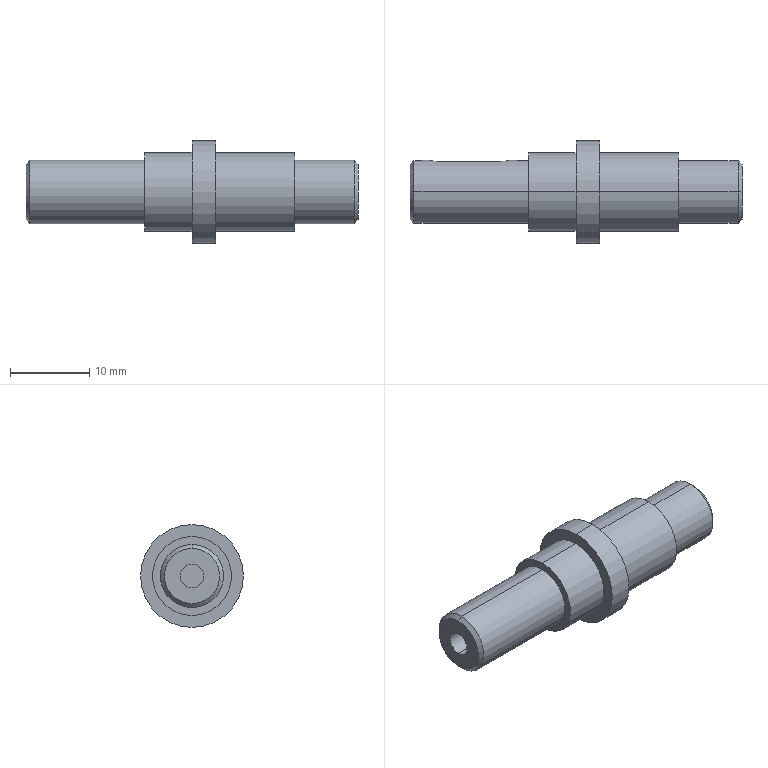Part | SolidWorks | features Chamfer 2, ICE 2, Revolution 1 | 1 solid | 28 faces | box 42 x 13 x 13 mm | volume 2716 mm3 | cylinder 14 | plane 10 | cone 4 | commonest cylinder face diameters 8 x4 10 x4 2 x2 3 x2 13 x2
STEP:
#1=CARTESIAN_POINT('',(18.732,0.,-3.5));
#2=VERTEX_POINT('',#1);
#3=CARTESIAN_POINT('',(18.732,0.,3.5));
#4=VERTEX_POINT('',#3);
#5=CARTESIAN_POINT('',(18.732,0.,0.));
#6=DIRECTION('',(1.,0.,0.));
#7=DIRECTION('',(0.,0.,1.));
#8=AXIS2_PLACEMENT_3D('',#5,#6,#7);
#9=CIRCLE('',#8,3.5);
#10=EDGE_CURVE('',#2,#4,#9,.T.);
#11=ORIENTED_EDGE('',*,*,#10,.F.);
#12=CARTESIAN_POINT('',(18.232,0.,-4.));
#13=VERTEX_POINT('',#12);
#14=CARTESIAN_POINT('',(18.232,0.,-4.));
#15=DIRECTION('',(-0.7071,0.,-0.7071));
#16=VECTOR('',#15,1000.);
#17=LINE('',#14,#16);
#18=EDGE_CURVE('',#2,#13,#17,.T.);
#19=ORIENTED_EDGE('',*,*,#18,.T.);
#20=CARTESIAN_POINT('',(18.232,0.,4.));
#21=VERTEX_POINT('',#20);
#22=CARTESIAN_POINT('',(18.232,0.,0.));
#23=DIRECTION('',(-1.,0.,0.));
#24=DIRECTION('',(0.,0.,1.));
#25=AXIS2_PLACEMENT_3D('',#22,#23,#24);
#26=CIRCLE('',#25,4.);
#27=EDGE_CURVE('',#21,#13,#26,.T.);
#28=ORIENTED_EDGE('',*,*,#27,.F.);
#29=CARTESIAN_POINT('',(18.232,0.,4.));
#30=DIRECTION('',(-0.7071,0.,0.7071));
#31=VECTOR('',#30,1000.);
#32=LINE('',#29,#31);
#33=EDGE_CURVE('',#4,#21,#32,.T.);
#34=ORIENTED_EDGE('',*,*,#33,.F.);
#35=EDGE_LOOP('',(#11,#19,#28,#34));
#36=FACE_OUTER_BOUND('',#35,.T.);
#37=CARTESIAN_POINT('',(18.232,0.,0.));
#38=DIRECTION('',(-1.,0.,0.));
#39=DIRECTION('',(0.,0.,1.));
#40=AXIS2_PLACEMENT_3D('',#37,#38,#39);
#41=CONICAL_SURFACE('',#40,4.,0.7854);
#42=ADVANCED_FACE('',(#36),#41,.T.);
#43=CARTESIAN_POINT('',(-23.268,0.,3.5));
#44=VERTEX_POINT('',#43);
#45=CARTESIAN_POINT('',(-23.268,0.,-3.5));
#46=VERTEX_POINT('',#45);
#47=CARTESIAN_POINT('',(-23.268,0.,0.));
#48=DIRECTION('',(-1.,0.,0.));
#49=DIRECTION('',(0.,0.,-1.));
#50=AXIS2_PLACEMENT_3D('',#47,#48,#49);
#51=CIRCLE('',#50,3.5);
#52=EDGE_CURVE('',#44,#46,#51,.T.);
#53=ORIENTED_EDGE('',*,*,#52,.F.);
#54=CARTESIAN_POINT('',(-22.768,0.,4.));
#55=VERTEX_POINT('',#54);
#56=CARTESIAN_POINT('',(-23.268,0.,3.5));
#57=DIRECTION('',(0.7071,0.,0.7071));
#58=VECTOR('',#57,1000.);
#59=LINE('',#56,#58);
#60=EDGE_CURVE('',#44,#55,#59,.T.);
#61=ORIENTED_EDGE('',*,*,#60,.T.);
#62=CARTESIAN_POINT('',(-22.768,0.,-4.));
#63=VERTEX_POINT('',#62);
#64=CARTESIAN_POINT('',(-22.768,0.,0.));
#65=DIRECTION('',(1.,0.,0.));
#66=DIRECTION('',(0.,0.,-1.));
#67=AXIS2_PLACEMENT_3D('',#64,#65,#66);
#68=CIRCLE('',#67,4.);
#69=EDGE_CURVE('',#63,#55,#68,.T.);
#70=ORIENTED_EDGE('',*,*,#69,.F.);
#71=CARTESIAN_POINT('',(-23.268,0.,-3.5));
#72=DIRECTION('',(0.7071,0.,-0.7071));
#73=VECTOR('',#72,1000.);
#74=LINE('',#71,#73);
#75=EDGE_CURVE('',#46,#63,#74,.T.);
#76=ORIENTED_EDGE('',*,*,#75,.F.);
#77=EDGE_LOOP('',(#53,#61,#70,#76));
#78=FACE_OUTER_BOUND('',#77,.T.);
#79=CARTESIAN_POINT('',(-23.268,0.,0.));
#80=DIRECTION('',(1.,0.,0.));
#81=DIRECTION('',(0.,0.,-1.));
#82=AXIS2_PLACEMENT_3D('',#79,#80,#81);
#83=CONICAL_SURFACE('',#82,3.5,0.7854);
#84=ADVANCED_FACE('',(#78),#83,.T.);
#85=CARTESIAN_POINT('',(-13.268,0.,-1.5));
#86=VERTEX_POINT('',#85);
#87=CARTESIAN_POINT('',(-13.268,0.,1.5));
#88=VERTEX_POINT('',#87);
#89=CARTESIAN_POINT('',(-13.268,0.,0.));
#90=DIRECTION('',(-1.,0.,0.));
#91=DIRECTION('',(0.,0.,1.));
#92=AXIS2_PLACEMENT_3D('',#89,#90,#91);
#93=CIRCLE('',#92,1.5);
#94=EDGE_CURVE('',#86,#88,#93,.T.);
#95=ORIENTED_EDGE('',*,*,#94,.F.);
#96=CARTESIAN_POINT('',(-23.268,0.,-1.5));
#97=VERTEX_POINT('',#96);
#98=CARTESIAN_POINT('',(-13.268,0.,-1.5));
#99=DIRECTION('',(-1.,0.,0.));
#100=VECTOR('',#99,1000.);
#101=LINE('',#98,#100);
#102=EDGE_CURVE('',#86,#97,#101,.T.);
#103=ORIENTED_EDGE('',*,*,#102,.T.);
#104=CARTESIAN_POINT('',(-23.268,0.,1.5));
#105=VERTEX_POINT('',#104);
#106=CARTESIAN_POINT('',(-23.268,0.,0.));
#107=DIRECTION('',(-1.,0.,0.));
#108=DIRECTION('',(0.,0.,1.));
#109=AXIS2_PLACEMENT_3D('',#106,#107,#108);
#110=CIRCLE('',#109,1.5);
#111=EDGE_CURVE('',#97,#105,#110,.T.);
#112=ORIENTED_EDGE('',*,*,#111,.T.);
#113=CARTESIAN_POINT('',(-13.268,0.,1.5));
#114=DIRECTION('',(-1.,0.,0.));
#115=VECTOR('',#114,1000.);
#116=LINE('',#113,#115);
#117=EDGE_CURVE('',#88,#105,#116,.T.);
#118=ORIENTED_EDGE('',*,*,#117,.F.);
#119=EDGE_LOOP('',(#95,#103,#112,#118));
#120=FACE_OUTER_BOUND('',#119,.T.);
#121=CARTESIAN_POINT('',(-13.268,0.,0.));
#122=DIRECTION('',(-1.,0.,0.));
#123=DIRECTION('',(0.,0.,1.));
#124=AXIS2_PLACEMENT_3D('',#121,#122,#123);
#125=CYLINDRICAL_SURFACE('',#124,1.5);
#126=ADVANCED_FACE('',(#120),#125,.F.);
#127=ORIENTED_EDGE('',*,*,#27,.T.);
#128=CARTESIAN_POINT('',(10.732,0.,-4.));
#129=VERTEX_POINT('',#128);
#130=CARTESIAN_POINT('',(-82.031,0.,-4.));
#131=DIRECTION('',(-1.,0.,0.));
#132=VECTOR('',#131,1000.);
#133=LINE('',#130,#132);
#134=EDGE_CURVE('',#13,#129,#133,.T.);
#135=ORIENTED_EDGE('',*,*,#134,.T.);
#136=CARTESIAN_POINT('',(10.732,0.,4.));
#137=VERTEX_POINT('',#136);
#138=CARTESIAN_POINT('',(10.732,0.,0.));
#139=DIRECTION('',(-1.,0.,0.));
#140=DIRECTION('',(0.,0.,1.));
#141=AXIS2_PLACEMENT_3D('',#138,#139,#140);
#142=CIRCLE('',#141,4.);
#143=EDGE_CURVE('',#137,#129,#142,.T.);
#144=ORIENTED_EDGE('',*,*,#143,.F.);
#145=CARTESIAN_POINT('',(-82.031,0.,4.));
#146=DIRECTION('',(-1.,0.,0.));
#147=VECTOR('',#146,1000.);
#148=LINE('',#145,#147);
#149=EDGE_CURVE('',#21,#137,#148,.T.);
#150=ORIENTED_EDGE('',*,*,#149,.F.);
#151=EDGE_LOOP('',(#127,#135,#144,#150));
#152=FACE_OUTER_BOUND('',#151,.T.);
#153=CARTESIAN_POINT('',(-82.031,0.,0.));
#154=DIRECTION('',(-1.,0.,0.));
#155=DIRECTION('',(0.,0.,1.));
#156=AXIS2_PLACEMENT_3D('',#153,#154,#155);
#157=CYLINDRICAL_SURFACE('',#156,4.);
#158=ADVANCED_FACE('',(#152),#157,.T.);
#159=CARTESIAN_POINT('',(10.732,0.,5.));
#160=VERTEX_POINT('',#159);
#161=CARTESIAN_POINT('',(10.732,0.,-5.));
#162=VERTEX_POINT('',#161);
#163=CARTESIAN_POINT('',(10.732,0.,0.));
#164=DIRECTION('',(-1.,0.,0.));
#165=DIRECTION('',(0.,0.,1.));
#166=AXIS2_PLACEMENT_3D('',#163,#164,#165);
#167=CIRCLE('',#166,5.);
#168=EDGE_CURVE('',#160,#162,#167,.T.);
#169=ORIENTED_EDGE('',*,*,#168,.T.);
#170=CARTESIAN_POINT('',(0.7324,0.,-5.));
#171=VERTEX_POINT('',#170);
#172=CARTESIAN_POINT('',(-82.031,0.,-5.));
#173=DIRECTION('',(-1.,0.,0.));
#174=VECTOR('',#173,1000.);
#175=LINE('',#172,#174);
#176=EDGE_CURVE('',#162,#171,#175,.T.);
#177=ORIENTED_EDGE('',*,*,#176,.T.);
#178=CARTESIAN_POINT('',(0.7324,0.,5.));
#179=VERTEX_POINT('',#178);
#180=CARTESIAN_POINT('',(0.7324,0.,0.));
#181=DIRECTION('',(-1.,0.,0.));
#182=DIRECTION('',(0.,0.,1.));
#183=AXIS2_PLACEMENT_3D('',#180,#181,#182);
#184=CIRCLE('',#183,5.);
#185=EDGE_CURVE('',#179,#171,#184,.T.);
#186=ORIENTED_EDGE('',*,*,#185,.F.);
#187=CARTESIAN_POINT('',(-82.031,0.,5.));
#188=DIRECTION('',(-1.,0.,0.));
#189=VECTOR('',#188,1000.);
#190=LINE('',#187,#189);
#191=EDGE_CURVE('',#160,#179,#190,.T.);
#192=ORIENTED_EDGE('',*,*,#191,.F.);
#193=EDGE_LOOP('',(#169,#177,#186,#192));
#194=FACE_OUTER_BOUND('',#193,.T.);
#195=CARTESIAN_POINT('',(-82.031,0.,0.));
#196=DIRECTION('',(-1.,0.,0.));
#197=DIRECTION('',(0.,0.,1.));
#198=AXIS2_PLACEMENT_3D('',#195,#196,#197);
#199=CYLINDRICAL_SURFACE('',#198,5.);
#200=ADVANCED_FACE('',(#194),#199,.T.);
#201=CARTESIAN_POINT('',(0.7324,0.,6.5));
#202=VERTEX_POINT('',#201);
#203=CARTESIAN_POINT('',(0.7324,0.,-6.5));
#204=VERTEX_POINT('',#203);
#205=CARTESIAN_POINT('',(0.7324,0.,0.));
#206=DIRECTION('',(-1.,0.,0.));
#207=DIRECTION('',(0.,0.,1.));
#208=AXIS2_PLACEMENT_3D('',#205,#206,#207);
#209=CIRCLE('',#208,6.5);
#210=EDGE_CURVE('',#202,#204,#209,.T.);
#211=ORIENTED_EDGE('',*,*,#210,.T.);
#212=CARTESIAN_POINT('',(-2.268,0.,-6.5));
#213=VERTEX_POINT('',#212);
#214=CARTESIAN_POINT('',(-82.031,0.,-6.5));
#215=DIRECTION('',(-1.,0.,0.));
#216=VECTOR('',#215,1000.);
#217=LINE('',#214,#216);
#218=EDGE_CURVE('',#204,#213,#217,.T.);
#219=ORIENTED_EDGE('',*,*,#218,.T.);
#220=CARTESIAN_POINT('',(-2.268,0.,6.5));
#221=VERTEX_POINT('',#220);
#222=CARTESIAN_POINT('',(-2.268,0.,0.));
#223=DIRECTION('',(-1.,0.,0.));
#224=DIRECTION('',(0.,0.,1.));
#225=AXIS2_PLACEMENT_3D('',#222,#223,#224);
#226=CIRCLE('',#225,6.5);
#227=EDGE_CURVE('',#221,#213,#226,.T.);
#228=ORIENTED_EDGE('',*,*,#227,.F.);
#229=CARTESIAN_POINT('',(-82.031,0.,6.5));
#230=DIRECTION('',(-1.,0.,0.));
#231=VECTOR('',#230,1000.);
#232=LINE('',#229,#231);
#233=EDGE_CURVE('',#202,#221,#232,.T.);
#234=ORIENTED_EDGE('',*,*,#233,.F.);
#235=EDGE_LOOP('',(#211,#219,#228,#234));
#236=FACE_OUTER_BOUND('',#235,.T.);
#237=CARTESIAN_POINT('',(-82.031,0.,0.));
#238=DIRECTION('',(-1.,0.,0.));
#239=DIRECTION('',(0.,0.,1.));
#240=AXIS2_PLACEMENT_3D('',#237,#238,#239);
#241=CYLINDRICAL_SURFACE('',#240,6.5);
#242=ADVANCED_FACE('',(#236),#241,.T.);
#243=CARTESIAN_POINT('',(-2.268,0.,5.));
#244=VERTEX_POINT('',#243);
#245=CARTESIAN_POINT('',(-2.268,0.,-5.));
#246=VERTEX_POINT('',#245);
#247=CARTESIAN_POINT('',(-2.268,0.,0.));
#248=DIRECTION('',(-1.,0.,0.));
#249=DIRECTION('',(0.,0.,1.));
#250=AXIS2_PLACEMENT_3D('',#247,#248,#249);
#251=CIRCLE('',#250,5.);
#252=EDGE_CURVE('',#244,#246,#251,.T.);
#253=ORIENTED_EDGE('',*,*,#252,.T.);
#254=CARTESIAN_POINT('',(-8.268,0.,-5.));
#255=VERTEX_POINT('',#254);
#256=CARTESIAN_POINT('',(-82.031,0.,-5.));
#257=DIRECTION('',(-1.,0.,0.));
#258=VECTOR('',#257,1000.);
#259=LINE('',#256,#258);
#260=EDGE_CURVE('',#246,#255,#259,.T.);
#261=ORIENTED_EDGE('',*,*,#260,.T.);
#262=CARTESIAN_POINT('',(-8.268,0.,5.));
#263=VERTEX_POINT('',#262);
#264=CARTESIAN_POINT('',(-8.268,0.,0.));
#265=DIRECTION('',(-1.,0.,0.));
#266=DIRECTION('',(0.,0.,1.));
#267=AXIS2_PLACEMENT_3D('',#264,#265,#266);
#268=CIRCLE('',#267,5.);
#269=EDGE_CURVE('',#263,#255,#268,.T.);
#270=ORIENTED_EDGE('',*,*,#269,.F.);
#271=CARTESIAN_POINT('',(-82.031,0.,5.));
#272=DIRECTION('',(-1.,0.,0.));
#273=VECTOR('',#272,1000.);
#274=LINE('',#271,#273);
#275=EDGE_CURVE('',#244,#263,#274,.T.);
#276=ORIENTED_EDGE('',*,*,#275,.F.);
#277=EDGE_LOOP('',(#253,#261,#270,#276));
#278=FACE_OUTER_BOUND('',#277,.T.);
#279=CARTESIAN_POINT('',(-82.031,0.,0.));
#280=DIRECTION('',(-1.,0.,0.));
#281=DIRECTION('',(0.,0.,1.));
#282=AXIS2_PLACEMENT_3D('',#279,#280,#281);
#283=CYLINDRICAL_SURFACE('',#282,5.);
#284=ADVANCED_FACE('',(#278),#283,.T.);
#285=CARTESIAN_POINT('',(-19.768,3.873,-1.));
#286=VERTEX_POINT('',#285);
#287=CARTESIAN_POINT('',(-11.768,3.873,-1.));
#288=VERTEX_POINT('',#287);
#289=CARTESIAN_POINT('',(-82.031,3.873,-1.));
#290=DIRECTION('',(1.,0.,0.));
#291=VECTOR('',#290,1000.);
#292=LINE('',#289,#291);
#293=EDGE_CURVE('',#286,#288,#292,.T.);
#294=ORIENTED_EDGE('',*,*,#293,.T.);
#295=CARTESIAN_POINT('',(-11.768,3.873,1.));
#296=VERTEX_POINT('',#295);
#297=CARTESIAN_POINT('',(-11.768,3.873,-1.));
#298=CARTESIAN_POINT('',(-11.635,3.873,-1.));
#299=CARTESIAN_POINT('',(-11.505,3.88,-0.9737));
#300=CARTESIAN_POINT('',(-11.263,3.904,-0.8732));
#301=CARTESIAN_POINT('',(-11.152,3.921,-0.7989));
#302=CARTESIAN_POINT('',(-10.969,3.953,-0.6153));
#303=CARTESIAN_POINT('',(-10.894,3.97,-0.5042));
#304=CARTESIAN_POINT('',(-10.794,3.993,-0.2638));
#305=CARTESIAN_POINT('',(-10.768,4.,-0.1319));
#306=CARTESIAN_POINT('',(-10.767,4.,0.1301));
#307=CARTESIAN_POINT('',(-10.793,3.993,0.2614));
#308=CARTESIAN_POINT('',(-10.894,3.97,0.5042));
#309=CARTESIAN_POINT('',(-10.968,3.954,0.6141));
#310=CARTESIAN_POINT('',(-11.153,3.92,0.7995));
#311=CARTESIAN_POINT('',(-11.263,3.904,0.8731));
#312=CARTESIAN_POINT('',(-11.504,3.88,0.9735));
#313=CARTESIAN_POINT('',(-11.635,3.873,1.));
#314=CARTESIAN_POINT('',(-11.768,3.873,1.));
#315=B_SPLINE_CURVE_WITH_KNOTS('',3,(#297,#298,#299,#300,#301,#302,#303,#304,#305,#306,#307,#308,#309,#310,#311,#312,#313,#314),.UNSPECIFIED.,.F.,.F.,(4,2,2,2,2,2,2,2,4),(0.,0.0003922,0.0007845,0.001177,0.001569,0.001961,0.002353,0.002746,0.003138),.UNSPECIFIED.);
#316=EDGE_CURVE('',#288,#296,#315,.T.);
#317=ORIENTED_EDGE('',*,*,#316,.T.);
#318=CARTESIAN_POINT('',(-19.768,3.873,1.));
#319=VERTEX_POINT('',#318);
#320=CARTESIAN_POINT('',(-82.031,3.873,1.));
#321=DIRECTION('',(-1.,0.,0.));
#322=VECTOR('',#321,1000.);
#323=LINE('',#320,#322);
#324=EDGE_CURVE('',#296,#319,#323,.T.);
#325=ORIENTED_EDGE('',*,*,#324,.T.);
#326=CARTESIAN_POINT('',(-19.768,3.873,1.));
#327=CARTESIAN_POINT('',(-19.9,3.873,1.));
#328=CARTESIAN_POINT('',(-20.03,3.88,0.9737));
#329=CARTESIAN_POINT('',(-20.272,3.904,0.8732));
#330=CARTESIAN_POINT('',(-20.383,3.921,0.7989));
#331=CARTESIAN_POINT('',(-20.566,3.953,0.6153));
#332=CARTESIAN_POINT('',(-20.641,3.97,0.5042));
#333=CARTESIAN_POINT('',(-20.741,3.993,0.2638));
#334=CARTESIAN_POINT('',(-20.767,4.,0.1319));
#335=CARTESIAN_POINT('',(-20.768,4.,-0.1301));
#336=CARTESIAN_POINT('',(-20.742,3.993,-0.2614));
#337=CARTESIAN_POINT('',(-20.641,3.97,-0.5042));
#338=CARTESIAN_POINT('',(-20.568,3.954,-0.6141));
#339=CARTESIAN_POINT('',(-20.382,3.92,-0.7995));
#340=CARTESIAN_POINT('',(-20.272,3.904,-0.8731));
#341=CARTESIAN_POINT('',(-20.031,3.88,-0.9735));
#342=CARTESIAN_POINT('',(-19.9,3.873,-1.));
#343=CARTESIAN_POINT('',(-19.768,3.873,-1.));
#344=B_SPLINE_CURVE_WITH_KNOTS('',3,(#326,#327,#328,#329,#330,#331,#332,#333,#334,#335,#336,#337,#338,#339,#340,#341,#342,#343),.UNSPECIFIED.,.F.,.F.,(4,2,2,2,2,2,2,2,4),(0.,0.0003922,0.0007845,0.001177,0.001569,0.001961,0.002353,0.002746,0.003138),.UNSPECIFIED.);
#345=EDGE_CURVE('',#319,#286,#344,.T.);
#346=ORIENTED_EDGE('',*,*,#345,.T.);
#347=EDGE_LOOP('',(#294,#317,#325,#346));
#348=FACE_BOUND('',#347,.T.);
#349=CARTESIAN_POINT('',(-8.268,0.,4.));
#350=VERTEX_POINT('',#349);
#351=CARTESIAN_POINT('',(-8.268,0.,-4.));
#352=VERTEX_POINT('',#351);
#353=CARTESIAN_POINT('',(-8.268,0.,0.));
#354=DIRECTION('',(-1.,0.,0.));
#355=DIRECTION('',(0.,0.,1.));
#356=AXIS2_PLACEMENT_3D('',#353,#354,#355);
#357=CIRCLE('',#356,4.);
#358=EDGE_CURVE('',#350,#352,#357,.T.);
#359=ORIENTED_EDGE('',*,*,#358,.T.);
#360=CARTESIAN_POINT('',(-82.031,0.,-4.));
#361=DIRECTION('',(-1.,0.,0.));
#362=VECTOR('',#361,1000.);
#363=LINE('',#360,#362);
#364=EDGE_CURVE('',#352,#63,#363,.T.);
#365=ORIENTED_EDGE('',*,*,#364,.T.);
#366=ORIENTED_EDGE('',*,*,#69,.T.);
#367=CARTESIAN_POINT('',(-82.031,0.,4.));
#368=DIRECTION('',(-1.,0.,0.));
#369=VECTOR('',#368,1000.);
#370=LINE('',#367,#369);
#371=EDGE_CURVE('',#350,#55,#370,.T.);
#372=ORIENTED_EDGE('',*,*,#371,.F.);
#373=EDGE_LOOP('',(#359,#365,#366,#372));
#374=FACE_OUTER_BOUND('',#373,.T.);
#375=CARTESIAN_POINT('',(-82.031,0.,0.));
#376=DIRECTION('',(-1.,0.,0.));
#377=DIRECTION('',(0.,0.,1.));
#378=AXIS2_PLACEMENT_3D('',#375,#376,#377);
#379=CYLINDRICAL_SURFACE('',#378,4.);
#380=ADVANCED_FACE('',(#348,#374),#379,.T.);
#381=CARTESIAN_POINT('',(-23.268,0.,0.));
#382=DIRECTION('',(-1.,0.,0.));
#383=DIRECTION('',(0.,0.,-1.));
#384=AXIS2_PLACEMENT_3D('',#381,#382,#383);
#385=CIRCLE('',#384,3.5);
#386=EDGE_CURVE('',#46,#44,#385,.T.);
#387=ORIENTED_EDGE('',*,*,#386,.T.);
#388=ORIENTED_EDGE('',*,*,#52,.T.);
#389=EDGE_LOOP('',(#387,#388));
#390=FACE_OUTER_BOUND('',#389,.T.);
#391=CARTESIAN_POINT('',(-23.268,0.,0.));
#392=DIRECTION('',(-1.,0.,0.));
#393=DIRECTION('',(0.,0.,1.));
#394=AXIS2_PLACEMENT_3D('',#391,#392,#393);
#395=CIRCLE('',#394,1.5);
#396=EDGE_CURVE('',#105,#97,#395,.T.);
#397=ORIENTED_EDGE('',*,*,#396,.F.);
#398=ORIENTED_EDGE('',*,*,#111,.F.);
#399=EDGE_LOOP('',(#397,#398));
#400=FACE_BOUND('',#399,.T.);
#401=CARTESIAN_POINT('',(-23.268,0.,0.));
#402=DIRECTION('',(1.,0.,0.));
#403=DIRECTION('',(0.,0.,-1.));
#404=AXIS2_PLACEMENT_3D('',#401,#402,#403);
#405=PLANE('',#404);
#406=ADVANCED_FACE('',(#390,#400),#405,.F.);
#407=ORIENTED_EDGE('',*,*,#364,.F.);
#408=CARTESIAN_POINT('',(-8.268,0.,0.));
#409=DIRECTION('',(-1.,0.,0.));
#410=DIRECTION('',(0.,0.,1.));
#411=AXIS2_PLACEMENT_3D('',#408,#409,#410);
#412=CIRCLE('',#411,4.);
#413=EDGE_CURVE('',#352,#350,#412,.T.);
#414=ORIENTED_EDGE('',*,*,#413,.T.);
#415=ORIENTED_EDGE('',*,*,#371,.T.);
#416=CARTESIAN_POINT('',(-22.768,0.,0.));
#417=DIRECTION('',(1.,0.,0.));
#418=DIRECTION('',(0.,0.,-1.));
#419=AXIS2_PLACEMENT_3D('',#416,#417,#418);
#420=CIRCLE('',#419,4.);
#421=EDGE_CURVE('',#55,#63,#420,.T.);
#422=ORIENTED_EDGE('',*,*,#421,.T.);
#423=EDGE_LOOP('',(#407,#414,#415,#422));
#424=FACE_OUTER_BOUND('',#423,.T.);
#425=CARTESIAN_POINT('',(-82.031,0.,0.));
#426=DIRECTION('',(-1.,0.,0.));
#427=DIRECTION('',(0.,0.,1.));
#428=AXIS2_PLACEMENT_3D('',#425,#426,#427);
#429=CYLINDRICAL_SURFACE('',#428,4.);
#430=ADVANCED_FACE('',(#424),#429,.T.);
#431=ORIENTED_EDGE('',*,*,#358,.F.);
#432=ORIENTED_EDGE('',*,*,#413,.F.);
#433=EDGE_LOOP('',(#431,#432));
#434=FACE_BOUND('',#433,.T.);
#435=ORIENTED_EDGE('',*,*,#269,.T.);
#436=CARTESIAN_POINT('',(-8.268,0.,0.));
#437=DIRECTION('',(-1.,0.,0.));
#438=DIRECTION('',(0.,0.,1.));
#439=AXIS2_PLACEMENT_3D('',#436,#437,#438);
#440=CIRCLE('',#439,5.);
#441=EDGE_CURVE('',#255,#263,#440,.T.);
#442=ORIENTED_EDGE('',*,*,#441,.T.);
#443=EDGE_LOOP('',(#435,#442));
#444=FACE_OUTER_BOUND('',#443,.T.);
#445=CARTESIAN_POINT('',(-8.268,4.,0.));
#446=DIRECTION('',(1.,0.,0.));
#447=DIRECTION('',(0.,0.,-1.));
#448=AXIS2_PLACEMENT_3D('',#445,#446,#447);
#449=PLANE('',#448);
#450=ADVANCED_FACE('',(#434,#444),#449,.F.);
#451=ORIENTED_EDGE('',*,*,#260,.F.);
#452=CARTESIAN_POINT('',(-2.268,0.,0.));
#453=DIRECTION('',(-1.,0.,0.));
#454=DIRECTION('',(0.,0.,1.));
#455=AXIS2_PLACEMENT_3D('',#452,#453,#454);
#456=CIRCLE('',#455,5.);
#457=EDGE_CURVE('',#246,#244,#456,.T.);
#458=ORIENTED_EDGE('',*,*,#457,.T.);
#459=ORIENTED_EDGE('',*,*,#275,.T.);
#460=ORIENTED_EDGE('',*,*,#441,.F.);
#461=EDGE_LOOP('',(#451,#458,#459,#460));
#462=FACE_OUTER_BOUND('',#461,.T.);
#463=CARTESIAN_POINT('',(-82.031,0.,0.));
#464=DIRECTION('',(-1.,0.,0.));
#465=DIRECTION('',(0.,0.,1.));
#466=AXIS2_PLACEMENT_3D('',#463,#464,#465);
#467=CYLINDRICAL_SURFACE('',#466,5.);
#468=ADVANCED_FACE('',(#462),#467,.T.);
#469=ORIENTED_EDGE('',*,*,#252,.F.);
#470=ORIENTED_EDGE('',*,*,#457,.F.);
#471=EDGE_LOOP('',(#469,#470));
#472=FACE_BOUND('',#471,.T.);
#473=ORIENTED_EDGE('',*,*,#227,.T.);
#474=CARTESIAN_POINT('',(-2.268,0.,0.));
#475=DIRECTION('',(-1.,0.,0.));
#476=DIRECTION('',(0.,0.,1.));
#477=AXIS2_PLACEMENT_3D('',#474,#475,#476);
#478=CIRCLE('',#477,6.5);
#479=EDGE_CURVE('',#213,#221,#478,.T.);
#480=ORIENTED_EDGE('',*,*,#479,.T.);
#481=EDGE_LOOP('',(#473,#480));
#482=FACE_OUTER_BOUND('',#481,.T.);
#483=CARTESIAN_POINT('',(-2.268,5.,0.));
#484=DIRECTION('',(1.,0.,0.));
#485=DIRECTION('',(0.,0.,-1.));
#486=AXIS2_PLACEMENT_3D('',#483,#484,#485);
#487=PLANE('',#486);
#488=ADVANCED_FACE('',(#472,#482),#487,.F.);
#489=ORIENTED_EDGE('',*,*,#218,.F.);
#490=CARTESIAN_POINT('',(0.7324,0.,0.));
#491=DIRECTION('',(-1.,0.,0.));
#492=DIRECTION('',(0.,0.,1.));
#493=AXIS2_PLACEMENT_3D('',#490,#491,#492);
#494=CIRCLE('',#493,6.5);
#495=EDGE_CURVE('',#204,#202,#494,.T.);
#496=ORIENTED_EDGE('',*,*,#495,.T.);
#497=ORIENTED_EDGE('',*,*,#233,.T.);
#498=ORIENTED_EDGE('',*,*,#479,.F.);
#499=EDGE_LOOP('',(#489,#496,#497,#498));
#500=FACE_OUTER_BOUND('',#499,.T.);
#501=CARTESIAN_POINT('',(-82.031,0.,0.));
#502=DIRECTION('',(-1.,0.,0.));
#503=DIRECTION('',(0.,0.,1.));
#504=AXIS2_PLACEMENT_3D('',#501,#502,#503);
#505=CYLINDRICAL_SURFACE('',#504,6.5);
#506=ADVANCED_FACE('',(#500),#505,.T.);
#507=ORIENTED_EDGE('',*,*,#210,.F.);
#508=ORIENTED_EDGE('',*,*,#495,.F.);
#509=EDGE_LOOP('',(#507,#508));
#510=FACE_OUTER_BOUND('',#509,.T.);
#511=ORIENTED_EDGE('',*,*,#185,.T.);
#512=CARTESIAN_POINT('',(0.7324,0.,0.));
#513=DIRECTION('',(-1.,0.,0.));
#514=DIRECTION('',(0.,0.,1.));
#515=AXIS2_PLACEMENT_3D('',#512,#513,#514);
#516=CIRCLE('',#515,5.);
#517=EDGE_CURVE('',#171,#179,#516,.T.);
#518=ORIENTED_EDGE('',*,*,#517,.T.);
#519=EDGE_LOOP('',(#511,#518));
#520=FACE_BOUND('',#519,.T.);
#521=CARTESIAN_POINT('',(0.7324,6.5,0.));
#522=DIRECTION('',(-1.,0.,0.));
#523=DIRECTION('',(0.,0.,1.));
#524=AXIS2_PLACEMENT_3D('',#521,#522,#523);
#525=PLANE('',#524);
#526=ADVANCED_FACE('',(#510,#520),#525,.F.);
#527=ORIENTED_EDGE('',*,*,#176,.F.);
#528=CARTESIAN_POINT('',(10.732,0.,0.));
#529=DIRECTION('',(-1.,0.,0.));
#530=DIRECTION('',(0.,0.,1.));
#531=AXIS2_PLACEMENT_3D('',#528,#529,#530);
#532=CIRCLE('',#531,5.);
#533=EDGE_CURVE('',#162,#160,#532,.T.);
#534=ORIENTED_EDGE('',*,*,#533,.T.);
#535=ORIENTED_EDGE('',*,*,#191,.T.);
#536=ORIENTED_EDGE('',*,*,#517,.F.);
#537=EDGE_LOOP('',(#527,#534,#535,#536));
#538=FACE_OUTER_BOUND('',#537,.T.);
#539=CARTESIAN_POINT('',(-82.031,0.,0.));
#540=DIRECTION('',(-1.,0.,0.));
#541=DIRECTION('',(0.,0.,1.));
#542=AXIS2_PLACEMENT_3D('',#539,#540,#541);
#543=CYLINDRICAL_SURFACE('',#542,5.);
#544=ADVANCED_FACE('',(#538),#543,.T.);
#545=ORIENTED_EDGE('',*,*,#168,.F.);
#546=ORIENTED_EDGE('',*,*,#533,.F.);
#547=EDGE_LOOP('',(#545,#546));
#548=FACE_OUTER_BOUND('',#547,.T.);
#549=ORIENTED_EDGE('',*,*,#143,.T.);
#550=CARTESIAN_POINT('',(10.732,0.,0.));
#551=DIRECTION('',(-1.,0.,0.));
#552=DIRECTION('',(0.,0.,1.));
#553=AXIS2_PLACEMENT_3D('',#550,#551,#552);
#554=CIRCLE('',#553,4.);
#555=EDGE_CURVE('',#129,#137,#554,.T.);
#556=ORIENTED_EDGE('',*,*,#555,.T.);
#557=EDGE_LOOP('',(#549,#556));
#558=FACE_BOUND('',#557,.T.);
#559=CARTESIAN_POINT('',(10.732,5.,0.));
#560=DIRECTION('',(-1.,0.,0.));
#561=DIRECTION('',(0.,0.,1.));
#562=AXIS2_PLACEMENT_3D('',#559,#560,#561);
#563=PLANE('',#562);
#564=ADVANCED_FACE('',(#548,#558),#563,.F.);
#565=ORIENTED_EDGE('',*,*,#134,.F.);
#566=CARTESIAN_POINT('',(18.232,0.,0.));
#567=DIRECTION('',(-1.,0.,0.));
#568=DIRECTION('',(0.,0.,1.));
#569=AXIS2_PLACEMENT_3D('',#566,#567,#568);
#570=CIRCLE('',#569,4.);
#571=EDGE_CURVE('',#13,#21,#570,.T.);
#572=ORIENTED_EDGE('',*,*,#571,.T.);
#573=ORIENTED_EDGE('',*,*,#149,.T.);
#574=ORIENTED_EDGE('',*,*,#555,.F.);
#575=EDGE_LOOP('',(#565,#572,#573,#574));
#576=FACE_OUTER_BOUND('',#575,.T.);
#577=CARTESIAN_POINT('',(-82.031,0.,0.));
#578=DIRECTION('',(-1.,0.,0.));
#579=DIRECTION('',(0.,0.,1.));
#580=AXIS2_PLACEMENT_3D('',#577,#578,#579);
#581=CYLINDRICAL_SURFACE('',#580,4.);
#582=ADVANCED_FACE('',(#576),#581,.T.);
#583=CARTESIAN_POINT('',(18.732,0.,0.));
#584=DIRECTION('',(1.,0.,0.));
#585=DIRECTION('',(0.,0.,1.));
#586=AXIS2_PLACEMENT_3D('',#583,#584,#585);
#587=CIRCLE('',#586,3.5);
#588=EDGE_CURVE('',#4,#2,#587,.T.);
#589=ORIENTED_EDGE('',*,*,#588,.T.);
#590=ORIENTED_EDGE('',*,*,#10,.T.);
#591=EDGE_LOOP('',(#589,#590));
#592=FACE_OUTER_BOUND('',#591,.T.);
#593=CARTESIAN_POINT('',(18.732,4.,0.));
#594=DIRECTION('',(-1.,0.,0.));
#595=DIRECTION('',(0.,0.,1.));
#596=AXIS2_PLACEMENT_3D('',#593,#594,#595);
#597=PLANE('',#596);
#598=ADVANCED_FACE('',(#592),#597,.F.);
#599=CARTESIAN_POINT('',(-19.768,3.,1.));
#600=VERTEX_POINT('',#599);
#601=CARTESIAN_POINT('',(-19.768,3.,1.));
#602=DIRECTION('',(0.,1.,0.));
#603=VECTOR('',#602,1000.);
#604=LINE('',#601,#603);
#605=EDGE_CURVE('',#600,#319,#604,.T.);
#606=ORIENTED_EDGE('',*,*,#605,.F.);
#607=CARTESIAN_POINT('',(-19.768,3.,-1.));
#608=VERTEX_POINT('',#607);
#609=CARTESIAN_POINT('',(-19.768,3.,0.));
#610=DIRECTION('',(0.,1.,0.));
#611=DIRECTION('',(0.,0.,1.));
#612=AXIS2_PLACEMENT_3D('',#609,#610,#611);
#613=CIRCLE('',#612,1.);
#614=EDGE_CURVE('',#608,#600,#613,.T.);
#615=ORIENTED_EDGE('',*,*,#614,.F.);
#616=CARTESIAN_POINT('',(-19.768,3.,-1.));
#617=DIRECTION('',(0.,1.,0.));
#618=VECTOR('',#617,1000.);
#619=LINE('',#616,#618);
#620=EDGE_CURVE('',#608,#286,#619,.T.);
#621=ORIENTED_EDGE('',*,*,#620,.T.);
#622=ORIENTED_EDGE('',*,*,#345,.F.);
#623=EDGE_LOOP('',(#606,#615,#621,#622));
#624=FACE_OUTER_BOUND('',#623,.T.);
#625=CARTESIAN_POINT('',(-19.768,3.,0.));
#626=DIRECTION('',(0.,1.,0.));
#627=DIRECTION('',(0.,0.,1.));
#628=AXIS2_PLACEMENT_3D('',#625,#626,#627);
#629=CYLINDRICAL_SURFACE('',#628,1.);
#630=ADVANCED_FACE('',(#624),#629,.F.);
#631=ORIENTED_EDGE('',*,*,#620,.F.);
#632=CARTESIAN_POINT('',(-11.768,3.,-1.));
#633=VERTEX_POINT('',#632);
#634=CARTESIAN_POINT('',(-19.768,3.,-1.));
#635=DIRECTION('',(-1.,0.,0.));
#636=VECTOR('',#635,1000.);
#637=LINE('',#634,#636);
#638=EDGE_CURVE('',#633,#608,#637,.T.);
#639=ORIENTED_EDGE('',*,*,#638,.F.);
#640=CARTESIAN_POINT('',(-11.768,3.,-1.));
#641=DIRECTION('',(0.,1.,0.));
#642=VECTOR('',#641,1000.);
#643=LINE('',#640,#642);
#644=EDGE_CURVE('',#633,#288,#643,.T.);
#645=ORIENTED_EDGE('',*,*,#644,.T.);
#646=ORIENTED_EDGE('',*,*,#293,.F.);
#647=EDGE_LOOP('',(#631,#639,#645,#646));
#648=FACE_OUTER_BOUND('',#647,.T.);
#649=CARTESIAN_POINT('',(-19.768,3.,-1.));
#650=DIRECTION('',(0.,0.,-1.));
#651=DIRECTION('',(-1.,0.,0.));
#652=AXIS2_PLACEMENT_3D('',#649,#650,#651);
#653=PLANE('',#652);
#654=ADVANCED_FACE('',(#648),#653,.F.);
#655=ORIENTED_EDGE('',*,*,#644,.F.);
#656=CARTESIAN_POINT('',(-11.768,3.,1.));
#657=VERTEX_POINT('',#656);
#658=CARTESIAN_POINT('',(-11.768,3.,0.));
#659=DIRECTION('',(0.,1.,0.));
#660=DIRECTION('',(0.,0.,1.));
#661=AXIS2_PLACEMENT_3D('',#658,#659,#660);
#662=CIRCLE('',#661,1.);
#663=EDGE_CURVE('',#657,#633,#662,.T.);
#664=ORIENTED_EDGE('',*,*,#663,.F.);
#665=CARTESIAN_POINT('',(-11.768,3.,1.));
#666=DIRECTION('',(0.,1.,0.));
#667=VECTOR('',#666,1000.);
#668=LINE('',#665,#667);
#669=EDGE_CURVE('',#657,#296,#668,.T.);
#670=ORIENTED_EDGE('',*,*,#669,.T.);
#671=ORIENTED_EDGE('',*,*,#316,.F.);
#672=EDGE_LOOP('',(#655,#664,#670,#671));
#673=FACE_OUTER_BOUND('',#672,.T.);
#674=CARTESIAN_POINT('',(-11.768,3.,0.));
#675=DIRECTION('',(0.,1.,0.));
#676=DIRECTION('',(0.,0.,1.));
#677=AXIS2_PLACEMENT_3D('',#674,#675,#676);
#678=CYLINDRICAL_SURFACE('',#677,1.);
#679=ADVANCED_FACE('',(#673),#678,.F.);
#680=ORIENTED_EDGE('',*,*,#669,.F.);
#681=CARTESIAN_POINT('',(-19.768,3.,1.));
#682=DIRECTION('',(1.,0.,0.));
#683=VECTOR('',#682,1000.);
#684=LINE('',#681,#683);
#685=EDGE_CURVE('',#600,#657,#684,.T.);
#686=ORIENTED_EDGE('',*,*,#685,.F.);
#687=ORIENTED_EDGE('',*,*,#605,.T.);
#688=ORIENTED_EDGE('',*,*,#324,.F.);
#689=EDGE_LOOP('',(#680,#686,#687,#688));
#690=FACE_OUTER_BOUND('',#689,.T.);
#691=CARTESIAN_POINT('',(-19.768,3.,1.));
#692=DIRECTION('',(0.,0.,1.));
#693=DIRECTION('',(1.,0.,0.));
#694=AXIS2_PLACEMENT_3D('',#691,#692,#693);
#695=PLANE('',#694);
#696=ADVANCED_FACE('',(#690),#695,.F.);
#697=ORIENTED_EDGE('',*,*,#614,.T.);
#698=ORIENTED_EDGE('',*,*,#685,.T.);
#699=ORIENTED_EDGE('',*,*,#663,.T.);
#700=ORIENTED_EDGE('',*,*,#638,.T.);
#701=EDGE_LOOP('',(#697,#698,#699,#700));
#702=FACE_OUTER_BOUND('',#701,.T.);
#703=CARTESIAN_POINT('',(-19.768,3.,0.));
#704=DIRECTION('',(0.,1.,0.));
#705=DIRECTION('',(0.,0.,1.));
#706=AXIS2_PLACEMENT_3D('',#703,#704,#705);
#707=PLANE('',#706);
#708=ADVANCED_FACE('',(#702),#707,.T.);
#709=ORIENTED_EDGE('',*,*,#102,.F.);
#710=CARTESIAN_POINT('',(-13.268,0.,0.));
#711=DIRECTION('',(-1.,0.,0.));
#712=DIRECTION('',(0.,0.,1.));
#713=AXIS2_PLACEMENT_3D('',#710,#711,#712);
#714=CIRCLE('',#713,1.5);
#715=EDGE_CURVE('',#88,#86,#714,.T.);
#716=ORIENTED_EDGE('',*,*,#715,.F.);
#717=ORIENTED_EDGE('',*,*,#117,.T.);
#718=ORIENTED_EDGE('',*,*,#396,.T.);
#719=EDGE_LOOP('',(#709,#716,#717,#718));
#720=FACE_OUTER_BOUND('',#719,.T.);
#721=CARTESIAN_POINT('',(-13.268,0.,0.));
#722=DIRECTION('',(-1.,0.,0.));
#723=DIRECTION('',(0.,0.,1.));
#724=AXIS2_PLACEMENT_3D('',#721,#722,#723);
#725=CYLINDRICAL_SURFACE('',#724,1.5);
#726=ADVANCED_FACE('',(#720),#725,.F.);
#727=ORIENTED_EDGE('',*,*,#715,.T.);
#728=ORIENTED_EDGE('',*,*,#94,.T.);
#729=EDGE_LOOP('',(#727,#728));
#730=FACE_OUTER_BOUND('',#729,.T.);
#731=CARTESIAN_POINT('',(-13.268,0.,0.));
#732=DIRECTION('',(-1.,0.,0.));
#733=DIRECTION('',(0.,0.,1.));
#734=AXIS2_PLACEMENT_3D('',#731,#732,#733);
#735=PLANE('',#734);
#736=ADVANCED_FACE('',(#730),#735,.T.);
#737=ORIENTED_EDGE('',*,*,#60,.F.);
#738=ORIENTED_EDGE('',*,*,#386,.F.);
#739=ORIENTED_EDGE('',*,*,#75,.T.);
#740=ORIENTED_EDGE('',*,*,#421,.F.);
#741=EDGE_LOOP('',(#737,#738,#739,#740));
#742=FACE_OUTER_BOUND('',#741,.T.);
#743=CARTESIAN_POINT('',(-23.268,0.,0.));
#744=DIRECTION('',(1.,0.,0.));
#745=DIRECTION('',(0.,0.,-1.));
#746=AXIS2_PLACEMENT_3D('',#743,#744,#745);
#747=CONICAL_SURFACE('',#746,3.5,0.7854);
#748=ADVANCED_FACE('',(#742),#747,.T.);
#749=ORIENTED_EDGE('',*,*,#18,.F.);
#750=ORIENTED_EDGE('',*,*,#588,.F.);
#751=ORIENTED_EDGE('',*,*,#33,.T.);
#752=ORIENTED_EDGE('',*,*,#571,.F.);
#753=EDGE_LOOP('',(#749,#750,#751,#752));
#754=FACE_OUTER_BOUND('',#753,.T.);
#755=CARTESIAN_POINT('',(18.232,0.,0.));
#756=DIRECTION('',(-1.,0.,0.));
#757=DIRECTION('',(0.,0.,1.));
#758=AXIS2_PLACEMENT_3D('',#755,#756,#757);
#759=CONICAL_SURFACE('',#758,4.,0.7854);
#760=ADVANCED_FACE('',(#754),#759,.T.);
#761=CLOSED_SHELL('',(#42,#84,#126,#158,#200,#242,#284,#380,#406,#430,#450,#468,#488,#506,#526,#544,#564,#582,#598,#630,#654,#679,#696,#708,#726,#736,#748,#760));
#762=MANIFOLD_SOLID_BREP('',#761);
#763=CARTESIAN_POINT('',(0.,0.,0.));
#764=DIRECTION('',(0.,0.,1.));
#765=DIRECTION('',(1.,0.,0.));
#766=AXIS2_PLACEMENT_3D('',#763,#764,#765);
#767=(LENGTH_UNIT()NAMED_UNIT(*)SI_UNIT(.MILLI.,.METRE.));
#768=UNCERTAINTY_MEASURE_WITH_UNIT(LENGTH_MEASURE(0.00001),#767,'','');
#769=(NAMED_UNIT(*)PLANE_ANGLE_UNIT()SI_UNIT($,.RADIAN.));
#770=(NAMED_UNIT(*)SI_UNIT($,.STERADIAN.)SOLID_ANGLE_UNIT());
#771=(GEOMETRIC_REPRESENTATION_CONTEXT(3)GLOBAL_UNCERTAINTY_ASSIGNED_CONTEXT((#768))GLOBAL_UNIT_ASSIGNED_CONTEXT((#767,#769,#770))REPRESENTATION_CONTEXT('',''));
#772=ADVANCED_BREP_SHAPE_REPRESENTATION('',(#762,#766),#771);